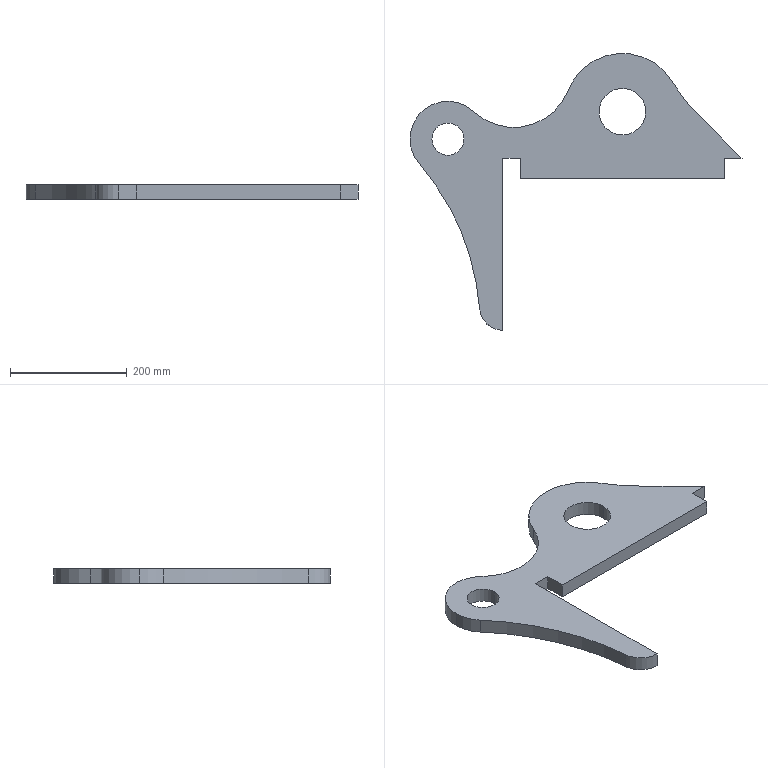Part | SolidWorks | features Extrusion 1 | 1 solid | 20 faces | box 569.4 x 475 x 25 mm | volume 2079428 mm3 | cylinder 11 | plane 9 | commonest cylinder face diameters 80 x3 55 x2 130 x2 200 x2 600 x1 860 x1
STEP:
#1=CARTESIAN_POINT('',(-326.8,-47.,25.));
#2=VERTEX_POINT('',#1);
#3=CARTESIAN_POINT('',(-271.8,-47.,25.));
#4=VERTEX_POINT('',#3);
#5=CARTESIAN_POINT('',(-299.3,-47.,25.));
#6=DIRECTION('',(0.,0.,1.));
#7=DIRECTION('',(1.,0.,0.));
#8=AXIS2_PLACEMENT_3D('',#5,#6,#7);
#9=CIRCLE('',#8,27.5);
#10=EDGE_CURVE('',#2,#4,#9,.T.);
#11=ORIENTED_EDGE('',*,*,#10,.T.);
#12=CARTESIAN_POINT('',(-271.8,-47.,0.));
#13=VERTEX_POINT('',#12);
#14=CARTESIAN_POINT('',(-271.8,-47.,25.));
#15=DIRECTION('',(0.,0.,-1.));
#16=VECTOR('',#15,1000.);
#17=LINE('',#14,#16);
#18=EDGE_CURVE('',#4,#13,#17,.T.);
#19=ORIENTED_EDGE('',*,*,#18,.T.);
#20=CARTESIAN_POINT('',(-326.8,-47.,0.));
#21=VERTEX_POINT('',#20);
#22=CARTESIAN_POINT('',(-299.3,-47.,0.));
#23=DIRECTION('',(0.,0.,1.));
#24=DIRECTION('',(1.,0.,0.));
#25=AXIS2_PLACEMENT_3D('',#22,#23,#24);
#26=CIRCLE('',#25,27.5);
#27=EDGE_CURVE('',#21,#13,#26,.T.);
#28=ORIENTED_EDGE('',*,*,#27,.F.);
#29=CARTESIAN_POINT('',(-326.8,-47.,25.));
#30=DIRECTION('',(0.,0.,-1.));
#31=VECTOR('',#30,1000.);
#32=LINE('',#29,#31);
#33=EDGE_CURVE('',#2,#21,#32,.T.);
#34=ORIENTED_EDGE('',*,*,#33,.F.);
#35=EDGE_LOOP('',(#11,#19,#28,#34));
#36=FACE_OUTER_BOUND('',#35,.T.);
#37=CARTESIAN_POINT('',(-299.3,-47.,25.));
#38=DIRECTION('',(0.,0.,-1.));
#39=DIRECTION('',(-1.,0.,0.));
#40=AXIS2_PLACEMENT_3D('',#37,#38,#39);
#41=CYLINDRICAL_SURFACE('',#40,27.5);
#42=ADVANCED_FACE('',(#36),#41,.F.);
#43=CARTESIAN_POINT('',(-40.,0.,25.));
#44=VERTEX_POINT('',#43);
#45=CARTESIAN_POINT('',(40.,0.,25.));
#46=VERTEX_POINT('',#45);
#47=CARTESIAN_POINT('',(0.,0.,25.));
#48=DIRECTION('',(0.,0.,1.));
#49=DIRECTION('',(1.,0.,0.));
#50=AXIS2_PLACEMENT_3D('',#47,#48,#49);
#51=CIRCLE('',#50,40.);
#52=EDGE_CURVE('',#44,#46,#51,.T.);
#53=ORIENTED_EDGE('',*,*,#52,.T.);
#54=CARTESIAN_POINT('',(40.,0.,0.));
#55=VERTEX_POINT('',#54);
#56=CARTESIAN_POINT('',(40.,0.,25.));
#57=DIRECTION('',(0.,0.,-1.));
#58=VECTOR('',#57,1000.);
#59=LINE('',#56,#58);
#60=EDGE_CURVE('',#46,#55,#59,.T.);
#61=ORIENTED_EDGE('',*,*,#60,.T.);
#62=CARTESIAN_POINT('',(-40.,0.,0.));
#63=VERTEX_POINT('',#62);
#64=CARTESIAN_POINT('',(0.,0.,0.));
#65=DIRECTION('',(0.,0.,1.));
#66=DIRECTION('',(1.,0.,0.));
#67=AXIS2_PLACEMENT_3D('',#64,#65,#66);
#68=CIRCLE('',#67,40.);
#69=EDGE_CURVE('',#63,#55,#68,.T.);
#70=ORIENTED_EDGE('',*,*,#69,.F.);
#71=CARTESIAN_POINT('',(-40.,0.,25.));
#72=DIRECTION('',(0.,0.,-1.));
#73=VECTOR('',#72,1000.);
#74=LINE('',#71,#73);
#75=EDGE_CURVE('',#44,#63,#74,.T.);
#76=ORIENTED_EDGE('',*,*,#75,.F.);
#77=EDGE_LOOP('',(#53,#61,#70,#76));
#78=FACE_OUTER_BOUND('',#77,.T.);
#79=CARTESIAN_POINT('',(0.,0.,25.));
#80=DIRECTION('',(0.,0.,-1.));
#81=DIRECTION('',(-1.,0.,0.));
#82=AXIS2_PLACEMENT_3D('',#79,#80,#81);
#83=CYLINDRICAL_SURFACE('',#82,40.);
#84=ADVANCED_FACE('',(#78),#83,.F.);
#85=CARTESIAN_POINT('',(-364.3,-47.,25.));
#86=VERTEX_POINT('',#85);
#87=CARTESIAN_POINT('',(-348.469,-89.514,25.));
#88=VERTEX_POINT('',#87);
#89=CARTESIAN_POINT('',(-299.3,-47.,25.));
#90=DIRECTION('',(0.,0.,1.));
#91=DIRECTION('',(1.,0.,0.));
#92=AXIS2_PLACEMENT_3D('',#89,#90,#91);
#93=CIRCLE('',#92,65.);
#94=EDGE_CURVE('',#86,#88,#93,.T.);
#95=ORIENTED_EDGE('',*,*,#94,.F.);
#96=CARTESIAN_POINT('',(-364.3,-47.,0.));
#97=VERTEX_POINT('',#96);
#98=CARTESIAN_POINT('',(-364.3,-47.,25.));
#99=DIRECTION('',(0.,0.,-1.));
#100=VECTOR('',#99,1000.);
#101=LINE('',#98,#100);
#102=EDGE_CURVE('',#86,#97,#101,.T.);
#103=ORIENTED_EDGE('',*,*,#102,.T.);
#104=CARTESIAN_POINT('',(-348.469,-89.514,0.));
#105=VERTEX_POINT('',#104);
#106=CARTESIAN_POINT('',(-299.3,-47.,0.));
#107=DIRECTION('',(0.,0.,1.));
#108=DIRECTION('',(1.,0.,0.));
#109=AXIS2_PLACEMENT_3D('',#106,#107,#108);
#110=CIRCLE('',#109,65.);
#111=EDGE_CURVE('',#97,#105,#110,.T.);
#112=ORIENTED_EDGE('',*,*,#111,.T.);
#113=CARTESIAN_POINT('',(-348.469,-89.514,25.));
#114=DIRECTION('',(0.,0.,-1.));
#115=VECTOR('',#114,1000.);
#116=LINE('',#113,#115);
#117=EDGE_CURVE('',#88,#105,#116,.T.);
#118=ORIENTED_EDGE('',*,*,#117,.F.);
#119=EDGE_LOOP('',(#95,#103,#112,#118));
#120=FACE_OUTER_BOUND('',#119,.T.);
#121=CARTESIAN_POINT('',(-299.3,-47.,25.));
#122=DIRECTION('',(0.,0.,-1.));
#123=DIRECTION('',(-1.,0.,0.));
#124=AXIS2_PLACEMENT_3D('',#121,#122,#123);
#125=CYLINDRICAL_SURFACE('',#124,65.);
#126=ADVANCED_FACE('',(#120),#125,.T.);
#127=ORIENTED_EDGE('',*,*,#52,.F.);
#128=CARTESIAN_POINT('',(0.,0.,25.));
#129=DIRECTION('',(0.,0.,1.));
#130=DIRECTION('',(1.,0.,0.));
#131=AXIS2_PLACEMENT_3D('',#128,#129,#130);
#132=CIRCLE('',#131,40.);
#133=EDGE_CURVE('',#46,#44,#132,.T.);
#134=ORIENTED_EDGE('',*,*,#133,.F.);
#135=EDGE_LOOP('',(#127,#134));
#136=FACE_BOUND('',#135,.T.);
#137=CARTESIAN_POINT('',(-175.1,-80.,25.));
#138=VERTEX_POINT('',#137);
#139=CARTESIAN_POINT('',(-175.1,-115.,25.));
#140=VERTEX_POINT('',#139);
#141=CARTESIAN_POINT('',(-175.1,-115.,25.));
#142=DIRECTION('',(0.,-1.,0.));
#143=VECTOR('',#142,1000.);
#144=LINE('',#141,#143);
#145=EDGE_CURVE('',#138,#140,#144,.T.);
#146=ORIENTED_EDGE('',*,*,#145,.T.);
#147=CARTESIAN_POINT('',(175.1,-115.,25.));
#148=VERTEX_POINT('',#147);
#149=CARTESIAN_POINT('',(-175.1,-115.,25.));
#150=DIRECTION('',(1.,0.,0.));
#151=VECTOR('',#150,1000.);
#152=LINE('',#149,#151);
#153=EDGE_CURVE('',#140,#148,#152,.T.);
#154=ORIENTED_EDGE('',*,*,#153,.T.);
#155=CARTESIAN_POINT('',(175.1,-80.,25.));
#156=VERTEX_POINT('',#155);
#157=CARTESIAN_POINT('',(175.1,-115.,25.));
#158=DIRECTION('',(0.,1.,0.));
#159=VECTOR('',#158,1000.);
#160=LINE('',#157,#159);
#161=EDGE_CURVE('',#148,#156,#160,.T.);
#162=ORIENTED_EDGE('',*,*,#161,.T.);
#163=CARTESIAN_POINT('',(205.1,-80.,25.));
#164=VERTEX_POINT('',#163);
#165=CARTESIAN_POINT('',(175.1,-80.,25.));
#166=DIRECTION('',(1.,0.,0.));
#167=VECTOR('',#166,1000.);
#168=LINE('',#165,#167);
#169=EDGE_CURVE('',#156,#164,#168,.T.);
#170=ORIENTED_EDGE('',*,*,#169,.T.);
#171=CARTESIAN_POINT('',(130.002,-4.902,25.));
#172=VERTEX_POINT('',#171);
#173=CARTESIAN_POINT('',(205.1,-80.,25.));
#174=DIRECTION('',(-0.7071,0.7071,0.));
#175=VECTOR('',#174,1000.);
#176=LINE('',#173,#175);
#177=EDGE_CURVE('',#164,#172,#176,.T.);
#178=ORIENTED_EDGE('',*,*,#177,.T.);
#179=CARTESIAN_POINT('',(85.534,51.807,25.));
#180=VERTEX_POINT('',#179);
#181=CARTESIAN_POINT('',(342.134,207.23,25.));
#182=DIRECTION('',(0.,0.,-1.));
#183=DIRECTION('',(1.,0.,0.));
#184=AXIS2_PLACEMENT_3D('',#181,#182,#183);
#185=CIRCLE('',#184,300.);
#186=EDGE_CURVE('',#172,#180,#185,.T.);
#187=ORIENTED_EDGE('',*,*,#186,.T.);
#188=CARTESIAN_POINT('',(-93.081,36.551,25.));
#189=VERTEX_POINT('',#188);
#190=CARTESIAN_POINT('',(0.,0.,25.));
#191=DIRECTION('',(0.,0.,1.));
#192=DIRECTION('',(1.,0.,0.));
#193=AXIS2_PLACEMENT_3D('',#190,#191,#192);
#194=CIRCLE('',#193,100.);
#195=EDGE_CURVE('',#180,#189,#194,.T.);
#196=ORIENTED_EDGE('',*,*,#195,.T.);
#197=CARTESIAN_POINT('',(-254.73,0.3131,25.));
#198=VERTEX_POINT('',#197);
#199=CARTESIAN_POINT('',(-186.161,73.103,25.));
#200=DIRECTION('',(0.,0.,-1.));
#201=DIRECTION('',(1.,0.,0.));
#202=AXIS2_PLACEMENT_3D('',#199,#200,#201);
#203=CIRCLE('',#202,100.);
#204=EDGE_CURVE('',#189,#198,#203,.T.);
#205=ORIENTED_EDGE('',*,*,#204,.T.);
#206=CARTESIAN_POINT('',(-299.3,-47.,25.));
#207=DIRECTION('',(0.,0.,1.));
#208=DIRECTION('',(1.,0.,0.));
#209=AXIS2_PLACEMENT_3D('',#206,#207,#208);
#210=CIRCLE('',#209,65.);
#211=EDGE_CURVE('',#198,#86,#210,.T.);
#212=ORIENTED_EDGE('',*,*,#211,.T.);
#213=ORIENTED_EDGE('',*,*,#94,.T.);
#214=CARTESIAN_POINT('',(-244.984,-338.044,25.));
#215=VERTEX_POINT('',#214);
#216=CARTESIAN_POINT('',(-673.738,-370.762,25.));
#217=DIRECTION('',(0.,0.,-1.));
#218=DIRECTION('',(1.,0.,0.));
#219=AXIS2_PLACEMENT_3D('',#216,#217,#218);
#220=CIRCLE('',#219,430.);
#221=EDGE_CURVE('',#88,#215,#220,.T.);
#222=ORIENTED_EDGE('',*,*,#221,.T.);
#223=CARTESIAN_POINT('',(-205.1,-375.,25.));
#224=VERTEX_POINT('',#223);
#225=CARTESIAN_POINT('',(-205.1,-335.,25.));
#226=DIRECTION('',(0.,0.,1.));
#227=DIRECTION('',(1.,0.,0.));
#228=AXIS2_PLACEMENT_3D('',#225,#226,#227);
#229=CIRCLE('',#228,40.);
#230=EDGE_CURVE('',#215,#224,#229,.T.);
#231=ORIENTED_EDGE('',*,*,#230,.T.);
#232=CARTESIAN_POINT('',(-205.1,-80.,25.));
#233=VERTEX_POINT('',#232);
#234=CARTESIAN_POINT('',(-205.1,-80.,25.));
#235=DIRECTION('',(0.,1.,0.));
#236=VECTOR('',#235,1000.);
#237=LINE('',#234,#236);
#238=EDGE_CURVE('',#224,#233,#237,.T.);
#239=ORIENTED_EDGE('',*,*,#238,.T.);
#240=CARTESIAN_POINT('',(-175.1,-80.,25.));
#241=DIRECTION('',(1.,0.,0.));
#242=VECTOR('',#241,1000.);
#243=LINE('',#240,#242);
#244=EDGE_CURVE('',#233,#138,#243,.T.);
#245=ORIENTED_EDGE('',*,*,#244,.T.);
#246=EDGE_LOOP('',(#146,#154,#162,#170,#178,#187,#196,#205,#212,#213,#222,#231,#239,#245));
#247=FACE_OUTER_BOUND('',#246,.T.);
#248=ORIENTED_EDGE('',*,*,#10,.F.);
#249=CARTESIAN_POINT('',(-299.3,-47.,25.));
#250=DIRECTION('',(0.,0.,1.));
#251=DIRECTION('',(1.,0.,0.));
#252=AXIS2_PLACEMENT_3D('',#249,#250,#251);
#253=CIRCLE('',#252,27.5);
#254=EDGE_CURVE('',#4,#2,#253,.T.);
#255=ORIENTED_EDGE('',*,*,#254,.F.);
#256=EDGE_LOOP('',(#248,#255));
#257=FACE_BOUND('',#256,.T.);
#258=CARTESIAN_POINT('',(-205.1,-335.,25.));
#259=DIRECTION('',(0.,0.,1.));
#260=DIRECTION('',(1.,0.,0.));
#261=AXIS2_PLACEMENT_3D('',#258,#259,#260);
#262=PLANE('',#261);
#263=ADVANCED_FACE('',(#136,#247,#257),#262,.T.);
#264=ORIENTED_EDGE('',*,*,#69,.T.);
#265=CARTESIAN_POINT('',(0.,0.,0.));
#266=DIRECTION('',(0.,0.,1.));
#267=DIRECTION('',(1.,0.,0.));
#268=AXIS2_PLACEMENT_3D('',#265,#266,#267);
#269=CIRCLE('',#268,40.);
#270=EDGE_CURVE('',#55,#63,#269,.T.);
#271=ORIENTED_EDGE('',*,*,#270,.T.);
#272=EDGE_LOOP('',(#264,#271));
#273=FACE_BOUND('',#272,.T.);
#274=CARTESIAN_POINT('',(-175.1,-80.,0.));
#275=VERTEX_POINT('',#274);
#276=CARTESIAN_POINT('',(-175.1,-115.,0.));
#277=VERTEX_POINT('',#276);
#278=CARTESIAN_POINT('',(-175.1,-115.,0.));
#279=DIRECTION('',(0.,-1.,0.));
#280=VECTOR('',#279,1000.);
#281=LINE('',#278,#280);
#282=EDGE_CURVE('',#275,#277,#281,.T.);
#283=ORIENTED_EDGE('',*,*,#282,.F.);
#284=CARTESIAN_POINT('',(-205.1,-80.,0.));
#285=VERTEX_POINT('',#284);
#286=CARTESIAN_POINT('',(-175.1,-80.,0.));
#287=DIRECTION('',(1.,0.,0.));
#288=VECTOR('',#287,1000.);
#289=LINE('',#286,#288);
#290=EDGE_CURVE('',#285,#275,#289,.T.);
#291=ORIENTED_EDGE('',*,*,#290,.F.);
#292=CARTESIAN_POINT('',(-205.1,-375.,0.));
#293=VERTEX_POINT('',#292);
#294=CARTESIAN_POINT('',(-205.1,-80.,0.));
#295=DIRECTION('',(0.,1.,0.));
#296=VECTOR('',#295,1000.);
#297=LINE('',#294,#296);
#298=EDGE_CURVE('',#293,#285,#297,.T.);
#299=ORIENTED_EDGE('',*,*,#298,.F.);
#300=CARTESIAN_POINT('',(-244.984,-338.044,0.));
#301=VERTEX_POINT('',#300);
#302=CARTESIAN_POINT('',(-205.1,-335.,0.));
#303=DIRECTION('',(0.,0.,1.));
#304=DIRECTION('',(1.,0.,0.));
#305=AXIS2_PLACEMENT_3D('',#302,#303,#304);
#306=CIRCLE('',#305,40.);
#307=EDGE_CURVE('',#301,#293,#306,.T.);
#308=ORIENTED_EDGE('',*,*,#307,.F.);
#309=CARTESIAN_POINT('',(-673.738,-370.762,0.));
#310=DIRECTION('',(0.,0.,-1.));
#311=DIRECTION('',(1.,0.,0.));
#312=AXIS2_PLACEMENT_3D('',#309,#310,#311);
#313=CIRCLE('',#312,430.);
#314=EDGE_CURVE('',#105,#301,#313,.T.);
#315=ORIENTED_EDGE('',*,*,#314,.F.);
#316=ORIENTED_EDGE('',*,*,#111,.F.);
#317=CARTESIAN_POINT('',(-254.73,0.3131,0.));
#318=VERTEX_POINT('',#317);
#319=CARTESIAN_POINT('',(-299.3,-47.,0.));
#320=DIRECTION('',(0.,0.,1.));
#321=DIRECTION('',(1.,0.,0.));
#322=AXIS2_PLACEMENT_3D('',#319,#320,#321);
#323=CIRCLE('',#322,65.);
#324=EDGE_CURVE('',#318,#97,#323,.T.);
#325=ORIENTED_EDGE('',*,*,#324,.F.);
#326=CARTESIAN_POINT('',(-93.081,36.551,0.));
#327=VERTEX_POINT('',#326);
#328=CARTESIAN_POINT('',(-186.161,73.103,0.));
#329=DIRECTION('',(0.,0.,-1.));
#330=DIRECTION('',(1.,0.,0.));
#331=AXIS2_PLACEMENT_3D('',#328,#329,#330);
#332=CIRCLE('',#331,100.);
#333=EDGE_CURVE('',#327,#318,#332,.T.);
#334=ORIENTED_EDGE('',*,*,#333,.F.);
#335=CARTESIAN_POINT('',(85.534,51.807,0.));
#336=VERTEX_POINT('',#335);
#337=CARTESIAN_POINT('',(0.,0.,0.));
#338=DIRECTION('',(0.,0.,1.));
#339=DIRECTION('',(1.,0.,0.));
#340=AXIS2_PLACEMENT_3D('',#337,#338,#339);
#341=CIRCLE('',#340,100.);
#342=EDGE_CURVE('',#336,#327,#341,.T.);
#343=ORIENTED_EDGE('',*,*,#342,.F.);
#344=CARTESIAN_POINT('',(130.002,-4.902,0.));
#345=VERTEX_POINT('',#344);
#346=CARTESIAN_POINT('',(342.134,207.23,0.));
#347=DIRECTION('',(0.,0.,-1.));
#348=DIRECTION('',(1.,0.,0.));
#349=AXIS2_PLACEMENT_3D('',#346,#347,#348);
#350=CIRCLE('',#349,300.);
#351=EDGE_CURVE('',#345,#336,#350,.T.);
#352=ORIENTED_EDGE('',*,*,#351,.F.);
#353=CARTESIAN_POINT('',(205.1,-80.,0.));
#354=VERTEX_POINT('',#353);
#355=CARTESIAN_POINT('',(205.1,-80.,0.));
#356=DIRECTION('',(-0.7071,0.7071,0.));
#357=VECTOR('',#356,1000.);
#358=LINE('',#355,#357);
#359=EDGE_CURVE('',#354,#345,#358,.T.);
#360=ORIENTED_EDGE('',*,*,#359,.F.);
#361=CARTESIAN_POINT('',(175.1,-80.,0.));
#362=VERTEX_POINT('',#361);
#363=CARTESIAN_POINT('',(175.1,-80.,0.));
#364=DIRECTION('',(1.,0.,0.));
#365=VECTOR('',#364,1000.);
#366=LINE('',#363,#365);
#367=EDGE_CURVE('',#362,#354,#366,.T.);
#368=ORIENTED_EDGE('',*,*,#367,.F.);
#369=CARTESIAN_POINT('',(175.1,-115.,0.));
#370=VERTEX_POINT('',#369);
#371=CARTESIAN_POINT('',(175.1,-115.,0.));
#372=DIRECTION('',(0.,1.,0.));
#373=VECTOR('',#372,1000.);
#374=LINE('',#371,#373);
#375=EDGE_CURVE('',#370,#362,#374,.T.);
#376=ORIENTED_EDGE('',*,*,#375,.F.);
#377=CARTESIAN_POINT('',(-175.1,-115.,0.));
#378=DIRECTION('',(1.,0.,0.));
#379=VECTOR('',#378,1000.);
#380=LINE('',#377,#379);
#381=EDGE_CURVE('',#277,#370,#380,.T.);
#382=ORIENTED_EDGE('',*,*,#381,.F.);
#383=EDGE_LOOP('',(#283,#291,#299,#308,#315,#316,#325,#334,#343,#352,#360,#368,#376,#382));
#384=FACE_OUTER_BOUND('',#383,.T.);
#385=ORIENTED_EDGE('',*,*,#27,.T.);
#386=CARTESIAN_POINT('',(-299.3,-47.,0.));
#387=DIRECTION('',(0.,0.,1.));
#388=DIRECTION('',(1.,0.,0.));
#389=AXIS2_PLACEMENT_3D('',#386,#387,#388);
#390=CIRCLE('',#389,27.5);
#391=EDGE_CURVE('',#13,#21,#390,.T.);
#392=ORIENTED_EDGE('',*,*,#391,.T.);
#393=EDGE_LOOP('',(#385,#392));
#394=FACE_BOUND('',#393,.T.);
#395=CARTESIAN_POINT('',(-205.1,-335.,0.));
#396=DIRECTION('',(0.,0.,1.));
#397=DIRECTION('',(1.,0.,0.));
#398=AXIS2_PLACEMENT_3D('',#395,#396,#397);
#399=PLANE('',#398);
#400=ADVANCED_FACE('',(#273,#384,#394),#399,.F.);
#401=ORIENTED_EDGE('',*,*,#282,.T.);
#402=CARTESIAN_POINT('',(-175.1,-115.,25.));
#403=DIRECTION('',(0.,0.,-1.));
#404=VECTOR('',#403,1000.);
#405=LINE('',#402,#404);
#406=EDGE_CURVE('',#140,#277,#405,.T.);
#407=ORIENTED_EDGE('',*,*,#406,.F.);
#408=ORIENTED_EDGE('',*,*,#145,.F.);
#409=CARTESIAN_POINT('',(-175.1,-80.,25.));
#410=DIRECTION('',(0.,0.,-1.));
#411=VECTOR('',#410,1000.);
#412=LINE('',#409,#411);
#413=EDGE_CURVE('',#138,#275,#412,.T.);
#414=ORIENTED_EDGE('',*,*,#413,.T.);
#415=EDGE_LOOP('',(#401,#407,#408,#414));
#416=FACE_OUTER_BOUND('',#415,.T.);
#417=CARTESIAN_POINT('',(-175.1,-115.,25.));
#418=DIRECTION('',(1.,0.,0.));
#419=DIRECTION('',(0.,0.,-1.));
#420=AXIS2_PLACEMENT_3D('',#417,#418,#419);
#421=PLANE('',#420);
#422=ADVANCED_FACE('',(#416),#421,.F.);
#423=ORIENTED_EDGE('',*,*,#381,.T.);
#424=CARTESIAN_POINT('',(175.1,-115.,25.));
#425=DIRECTION('',(0.,0.,-1.));
#426=VECTOR('',#425,1000.);
#427=LINE('',#424,#426);
#428=EDGE_CURVE('',#148,#370,#427,.T.);
#429=ORIENTED_EDGE('',*,*,#428,.F.);
#430=ORIENTED_EDGE('',*,*,#153,.F.);
#431=ORIENTED_EDGE('',*,*,#406,.T.);
#432=EDGE_LOOP('',(#423,#429,#430,#431));
#433=FACE_OUTER_BOUND('',#432,.T.);
#434=CARTESIAN_POINT('',(-175.1,-115.,25.));
#435=DIRECTION('',(0.,1.,0.));
#436=DIRECTION('',(-1.,0.,0.));
#437=AXIS2_PLACEMENT_3D('',#434,#435,#436);
#438=PLANE('',#437);
#439=ADVANCED_FACE('',(#433),#438,.F.);
#440=ORIENTED_EDGE('',*,*,#375,.T.);
#441=CARTESIAN_POINT('',(175.1,-80.,25.));
#442=DIRECTION('',(0.,0.,-1.));
#443=VECTOR('',#442,1000.);
#444=LINE('',#441,#443);
#445=EDGE_CURVE('',#156,#362,#444,.T.);
#446=ORIENTED_EDGE('',*,*,#445,.F.);
#447=ORIENTED_EDGE('',*,*,#161,.F.);
#448=ORIENTED_EDGE('',*,*,#428,.T.);
#449=EDGE_LOOP('',(#440,#446,#447,#448));
#450=FACE_OUTER_BOUND('',#449,.T.);
#451=CARTESIAN_POINT('',(175.1,-115.,25.));
#452=DIRECTION('',(-1.,0.,0.));
#453=DIRECTION('',(0.,0.,1.));
#454=AXIS2_PLACEMENT_3D('',#451,#452,#453);
#455=PLANE('',#454);
#456=ADVANCED_FACE('',(#450),#455,.F.);
#457=ORIENTED_EDGE('',*,*,#367,.T.);
#458=CARTESIAN_POINT('',(205.1,-80.,25.));
#459=DIRECTION('',(0.,0.,-1.));
#460=VECTOR('',#459,1000.);
#461=LINE('',#458,#460);
#462=EDGE_CURVE('',#164,#354,#461,.T.);
#463=ORIENTED_EDGE('',*,*,#462,.F.);
#464=ORIENTED_EDGE('',*,*,#169,.F.);
#465=ORIENTED_EDGE('',*,*,#445,.T.);
#466=EDGE_LOOP('',(#457,#463,#464,#465));
#467=FACE_OUTER_BOUND('',#466,.T.);
#468=CARTESIAN_POINT('',(175.1,-80.,25.));
#469=DIRECTION('',(0.,1.,0.));
#470=DIRECTION('',(0.,0.,1.));
#471=AXIS2_PLACEMENT_3D('',#468,#469,#470);
#472=PLANE('',#471);
#473=ADVANCED_FACE('',(#467),#472,.F.);
#474=ORIENTED_EDGE('',*,*,#359,.T.);
#475=CARTESIAN_POINT('',(130.002,-4.902,25.));
#476=DIRECTION('',(0.,0.,-1.));
#477=VECTOR('',#476,1000.);
#478=LINE('',#475,#477);
#479=EDGE_CURVE('',#172,#345,#478,.T.);
#480=ORIENTED_EDGE('',*,*,#479,.F.);
#481=ORIENTED_EDGE('',*,*,#177,.F.);
#482=ORIENTED_EDGE('',*,*,#462,.T.);
#483=EDGE_LOOP('',(#474,#480,#481,#482));
#484=FACE_OUTER_BOUND('',#483,.T.);
#485=CARTESIAN_POINT('',(205.1,-80.,25.));
#486=DIRECTION('',(-0.7071,-0.7071,0.));
#487=DIRECTION('',(0.7071,-0.7071,0.));
#488=AXIS2_PLACEMENT_3D('',#485,#486,#487);
#489=PLANE('',#488);
#490=ADVANCED_FACE('',(#484),#489,.F.);
#491=ORIENTED_EDGE('',*,*,#351,.T.);
#492=CARTESIAN_POINT('',(85.534,51.807,25.));
#493=DIRECTION('',(0.,0.,-1.));
#494=VECTOR('',#493,1000.);
#495=LINE('',#492,#494);
#496=EDGE_CURVE('',#180,#336,#495,.T.);
#497=ORIENTED_EDGE('',*,*,#496,.F.);
#498=ORIENTED_EDGE('',*,*,#186,.F.);
#499=ORIENTED_EDGE('',*,*,#479,.T.);
#500=EDGE_LOOP('',(#491,#497,#498,#499));
#501=FACE_OUTER_BOUND('',#500,.T.);
#502=CARTESIAN_POINT('',(342.134,207.23,25.));
#503=DIRECTION('',(0.,0.,-1.));
#504=DIRECTION('',(-1.,0.,0.));
#505=AXIS2_PLACEMENT_3D('',#502,#503,#504);
#506=CYLINDRICAL_SURFACE('',#505,300.);
#507=ADVANCED_FACE('',(#501),#506,.F.);
#508=ORIENTED_EDGE('',*,*,#342,.T.);
#509=CARTESIAN_POINT('',(-93.081,36.551,25.));
#510=DIRECTION('',(0.,0.,-1.));
#511=VECTOR('',#510,1000.);
#512=LINE('',#509,#511);
#513=EDGE_CURVE('',#189,#327,#512,.T.);
#514=ORIENTED_EDGE('',*,*,#513,.F.);
#515=ORIENTED_EDGE('',*,*,#195,.F.);
#516=ORIENTED_EDGE('',*,*,#496,.T.);
#517=EDGE_LOOP('',(#508,#514,#515,#516));
#518=FACE_OUTER_BOUND('',#517,.T.);
#519=CARTESIAN_POINT('',(0.,0.,25.));
#520=DIRECTION('',(0.,0.,-1.));
#521=DIRECTION('',(-1.,0.,0.));
#522=AXIS2_PLACEMENT_3D('',#519,#520,#521);
#523=CYLINDRICAL_SURFACE('',#522,100.);
#524=ADVANCED_FACE('',(#518),#523,.T.);
#525=ORIENTED_EDGE('',*,*,#333,.T.);
#526=CARTESIAN_POINT('',(-254.73,0.3131,25.));
#527=DIRECTION('',(0.,0.,-1.));
#528=VECTOR('',#527,1000.);
#529=LINE('',#526,#528);
#530=EDGE_CURVE('',#198,#318,#529,.T.);
#531=ORIENTED_EDGE('',*,*,#530,.F.);
#532=ORIENTED_EDGE('',*,*,#204,.F.);
#533=ORIENTED_EDGE('',*,*,#513,.T.);
#534=EDGE_LOOP('',(#525,#531,#532,#533));
#535=FACE_OUTER_BOUND('',#534,.T.);
#536=CARTESIAN_POINT('',(-186.161,73.103,25.));
#537=DIRECTION('',(0.,0.,-1.));
#538=DIRECTION('',(-1.,0.,0.));
#539=AXIS2_PLACEMENT_3D('',#536,#537,#538);
#540=CYLINDRICAL_SURFACE('',#539,100.);
#541=ADVANCED_FACE('',(#535),#540,.F.);
#542=ORIENTED_EDGE('',*,*,#102,.F.);
#543=ORIENTED_EDGE('',*,*,#211,.F.);
#544=ORIENTED_EDGE('',*,*,#530,.T.);
#545=ORIENTED_EDGE('',*,*,#324,.T.);
#546=EDGE_LOOP('',(#542,#543,#544,#545));
#547=FACE_OUTER_BOUND('',#546,.T.);
#548=CARTESIAN_POINT('',(-299.3,-47.,25.));
#549=DIRECTION('',(0.,0.,-1.));
#550=DIRECTION('',(-1.,0.,0.));
#551=AXIS2_PLACEMENT_3D('',#548,#549,#550);
#552=CYLINDRICAL_SURFACE('',#551,65.);
#553=ADVANCED_FACE('',(#547),#552,.T.);
#554=ORIENTED_EDGE('',*,*,#314,.T.);
#555=CARTESIAN_POINT('',(-244.984,-338.044,25.));
#556=DIRECTION('',(0.,0.,-1.));
#557=VECTOR('',#556,1000.);
#558=LINE('',#555,#557);
#559=EDGE_CURVE('',#215,#301,#558,.T.);
#560=ORIENTED_EDGE('',*,*,#559,.F.);
#561=ORIENTED_EDGE('',*,*,#221,.F.);
#562=ORIENTED_EDGE('',*,*,#117,.T.);
#563=EDGE_LOOP('',(#554,#560,#561,#562));
#564=FACE_OUTER_BOUND('',#563,.T.);
#565=CARTESIAN_POINT('',(-673.738,-370.762,25.));
#566=DIRECTION('',(0.,0.,-1.));
#567=DIRECTION('',(-1.,0.,0.));
#568=AXIS2_PLACEMENT_3D('',#565,#566,#567);
#569=CYLINDRICAL_SURFACE('',#568,430.);
#570=ADVANCED_FACE('',(#564),#569,.F.);
#571=ORIENTED_EDGE('',*,*,#307,.T.);
#572=CARTESIAN_POINT('',(-205.1,-375.,25.));
#573=DIRECTION('',(0.,0.,-1.));
#574=VECTOR('',#573,1000.);
#575=LINE('',#572,#574);
#576=EDGE_CURVE('',#224,#293,#575,.T.);
#577=ORIENTED_EDGE('',*,*,#576,.F.);
#578=ORIENTED_EDGE('',*,*,#230,.F.);
#579=ORIENTED_EDGE('',*,*,#559,.T.);
#580=EDGE_LOOP('',(#571,#577,#578,#579));
#581=FACE_OUTER_BOUND('',#580,.T.);
#582=CARTESIAN_POINT('',(-205.1,-335.,25.));
#583=DIRECTION('',(0.,0.,-1.));
#584=DIRECTION('',(-1.,0.,0.));
#585=AXIS2_PLACEMENT_3D('',#582,#583,#584);
#586=CYLINDRICAL_SURFACE('',#585,40.);
#587=ADVANCED_FACE('',(#581),#586,.T.);
#588=ORIENTED_EDGE('',*,*,#298,.T.);
#589=CARTESIAN_POINT('',(-205.1,-80.,25.));
#590=DIRECTION('',(0.,0.,-1.));
#591=VECTOR('',#590,1000.);
#592=LINE('',#589,#591);
#593=EDGE_CURVE('',#233,#285,#592,.T.);
#594=ORIENTED_EDGE('',*,*,#593,.F.);
#595=ORIENTED_EDGE('',*,*,#238,.F.);
#596=ORIENTED_EDGE('',*,*,#576,.T.);
#597=EDGE_LOOP('',(#588,#594,#595,#596));
#598=FACE_OUTER_BOUND('',#597,.T.);
#599=CARTESIAN_POINT('',(-205.1,-80.,25.));
#600=DIRECTION('',(-1.,0.,0.));
#601=DIRECTION('',(0.,-1.,0.));
#602=AXIS2_PLACEMENT_3D('',#599,#600,#601);
#603=PLANE('',#602);
#604=ADVANCED_FACE('',(#598),#603,.F.);
#605=ORIENTED_EDGE('',*,*,#290,.T.);
#606=ORIENTED_EDGE('',*,*,#413,.F.);
#607=ORIENTED_EDGE('',*,*,#244,.F.);
#608=ORIENTED_EDGE('',*,*,#593,.T.);
#609=EDGE_LOOP('',(#605,#606,#607,#608));
#610=FACE_OUTER_BOUND('',#609,.T.);
#611=CARTESIAN_POINT('',(-175.1,-80.,25.));
#612=DIRECTION('',(0.,1.,0.));
#613=DIRECTION('',(0.,0.,1.));
#614=AXIS2_PLACEMENT_3D('',#611,#612,#613);
#615=PLANE('',#614);
#616=ADVANCED_FACE('',(#610),#615,.F.);
#617=ORIENTED_EDGE('',*,*,#60,.F.);
#618=ORIENTED_EDGE('',*,*,#133,.T.);
#619=ORIENTED_EDGE('',*,*,#75,.T.);
#620=ORIENTED_EDGE('',*,*,#270,.F.);
#621=EDGE_LOOP('',(#617,#618,#619,#620));
#622=FACE_OUTER_BOUND('',#621,.T.);
#623=CARTESIAN_POINT('',(0.,0.,25.));
#624=DIRECTION('',(0.,0.,-1.));
#625=DIRECTION('',(-1.,0.,0.));
#626=AXIS2_PLACEMENT_3D('',#623,#624,#625);
#627=CYLINDRICAL_SURFACE('',#626,40.);
#628=ADVANCED_FACE('',(#622),#627,.F.);
#629=ORIENTED_EDGE('',*,*,#18,.F.);
#630=ORIENTED_EDGE('',*,*,#254,.T.);
#631=ORIENTED_EDGE('',*,*,#33,.T.);
#632=ORIENTED_EDGE('',*,*,#391,.F.);
#633=EDGE_LOOP('',(#629,#630,#631,#632));
#634=FACE_OUTER_BOUND('',#633,.T.);
#635=CARTESIAN_POINT('',(-299.3,-47.,25.));
#636=DIRECTION('',(0.,0.,-1.));
#637=DIRECTION('',(-1.,0.,0.));
#638=AXIS2_PLACEMENT_3D('',#635,#636,#637);
#639=CYLINDRICAL_SURFACE('',#638,27.5);
#640=ADVANCED_FACE('',(#634),#639,.F.);
#641=CLOSED_SHELL('',(#42,#84,#126,#263,#400,#422,#439,#456,#473,#490,#507,#524,#541,#553,#570,#587,#604,#616,#628,#640));
#642=MANIFOLD_SOLID_BREP('',#641);
#643=CARTESIAN_POINT('',(0.,0.,0.));
#644=DIRECTION('',(0.,0.,1.));
#645=DIRECTION('',(1.,0.,0.));
#646=AXIS2_PLACEMENT_3D('',#643,#644,#645);
#647=(LENGTH_UNIT()NAMED_UNIT(*)SI_UNIT(.MILLI.,.METRE.));
#648=UNCERTAINTY_MEASURE_WITH_UNIT(LENGTH_MEASURE(0.00001),#647,'','');
#649=(NAMED_UNIT(*)PLANE_ANGLE_UNIT()SI_UNIT($,.RADIAN.));
#650=(NAMED_UNIT(*)SI_UNIT($,.STERADIAN.)SOLID_ANGLE_UNIT());
#651=(GEOMETRIC_REPRESENTATION_CONTEXT(3)GLOBAL_UNCERTAINTY_ASSIGNED_CONTEXT((#648))GLOBAL_UNIT_ASSIGNED_CONTEXT((#647,#649,#650))REPRESENTATION_CONTEXT('',''));
#652=ADVANCED_BREP_SHAPE_REPRESENTATION('',(#642,#646),#651);